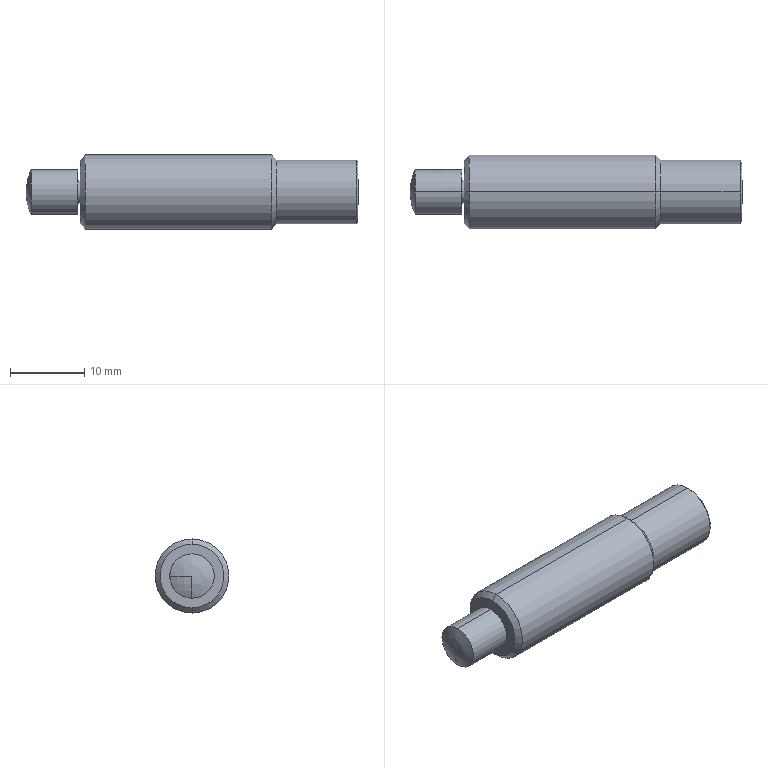Part | STEP file | P649654_YSRT_7_5_C | 1 solid | 26 faces | box 44.8 x 10 x 10 mm | volume 2880 mm3 | plane 10 | cylinder 8 | cone 6 | spline 2 | commonest cylinder face diameters 3 x2 6 x2 8.6 x2 10 x2